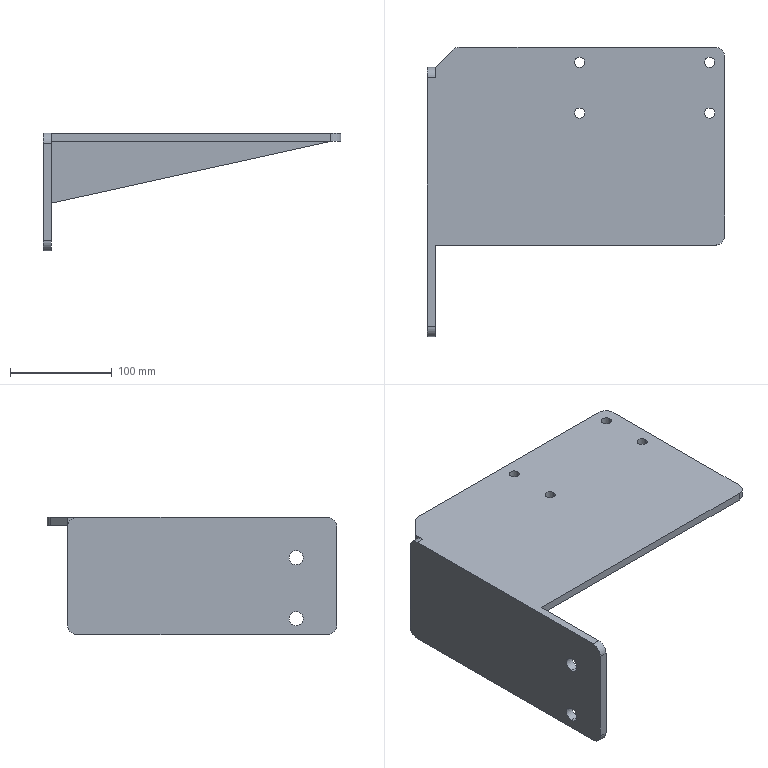Part | SolidWorks | features BaseBody 2 | 2 solids | 36 faces | box 293 x 285 x 116 mm | volume 750279 mm3 | cylinder 19 | plane 17 | commonest cylinder face diameters 10 x8 20 x7 14 x4
STEP:
#1=CARTESIAN_POINT('',(8.,40.,23.));
#2=VERTEX_POINT('',#1);
#3=CARTESIAN_POINT('',(8.,40.,9.));
#4=VERTEX_POINT('',#3);
#5=CARTESIAN_POINT('',(8.,40.,16.));
#6=DIRECTION('',(1.,0.,0.));
#7=DIRECTION('',(0.,1.,0.));
#8=AXIS2_PLACEMENT_3D('',#5,#6,#7);
#9=CIRCLE('',#8,7.);
#10=EDGE_CURVE('',#2,#4,#9,.T.);
#11=ORIENTED_EDGE('',*,*,#10,.T.);
#12=CARTESIAN_POINT('',(0.,40.,9.));
#13=VERTEX_POINT('',#12);
#14=CARTESIAN_POINT('',(8.,40.,9.));
#15=DIRECTION('',(-1.,0.,0.));
#16=VECTOR('',#15,1000.);
#17=LINE('',#14,#16);
#18=EDGE_CURVE('',#4,#13,#17,.T.);
#19=ORIENTED_EDGE('',*,*,#18,.T.);
#20=CARTESIAN_POINT('',(0.,40.,23.));
#21=VERTEX_POINT('',#20);
#22=CARTESIAN_POINT('',(0.,40.,16.));
#23=DIRECTION('',(1.,0.,0.));
#24=DIRECTION('',(0.,1.,0.));
#25=AXIS2_PLACEMENT_3D('',#22,#23,#24);
#26=CIRCLE('',#25,7.);
#27=EDGE_CURVE('',#21,#13,#26,.T.);
#28=ORIENTED_EDGE('',*,*,#27,.F.);
#29=CARTESIAN_POINT('',(8.,40.,23.));
#30=DIRECTION('',(-1.,0.,0.));
#31=VECTOR('',#30,1000.);
#32=LINE('',#29,#31);
#33=EDGE_CURVE('',#2,#21,#32,.T.);
#34=ORIENTED_EDGE('',*,*,#33,.F.);
#35=EDGE_LOOP('',(#11,#19,#28,#34));
#36=FACE_OUTER_BOUND('',#35,.T.);
#37=CARTESIAN_POINT('',(8.,40.,16.));
#38=DIRECTION('',(-1.,0.,0.));
#39=DIRECTION('',(0.,0.,1.));
#40=AXIS2_PLACEMENT_3D('',#37,#38,#39);
#41=CYLINDRICAL_SURFACE('',#40,7.);
#42=ADVANCED_FACE('',(#36),#41,.F.);
#43=CARTESIAN_POINT('',(8.,40.,83.));
#44=VERTEX_POINT('',#43);
#45=CARTESIAN_POINT('',(8.,40.,69.));
#46=VERTEX_POINT('',#45);
#47=CARTESIAN_POINT('',(8.,40.,76.));
#48=DIRECTION('',(1.,0.,0.));
#49=DIRECTION('',(0.,1.,0.));
#50=AXIS2_PLACEMENT_3D('',#47,#48,#49);
#51=CIRCLE('',#50,7.);
#52=EDGE_CURVE('',#44,#46,#51,.T.);
#53=ORIENTED_EDGE('',*,*,#52,.T.);
#54=CARTESIAN_POINT('',(0.,40.,69.));
#55=VERTEX_POINT('',#54);
#56=CARTESIAN_POINT('',(8.,40.,69.));
#57=DIRECTION('',(-1.,0.,0.));
#58=VECTOR('',#57,1000.);
#59=LINE('',#56,#58);
#60=EDGE_CURVE('',#46,#55,#59,.T.);
#61=ORIENTED_EDGE('',*,*,#60,.T.);
#62=CARTESIAN_POINT('',(0.,40.,83.));
#63=VERTEX_POINT('',#62);
#64=CARTESIAN_POINT('',(0.,40.,76.));
#65=DIRECTION('',(1.,0.,0.));
#66=DIRECTION('',(0.,1.,0.));
#67=AXIS2_PLACEMENT_3D('',#64,#65,#66);
#68=CIRCLE('',#67,7.);
#69=EDGE_CURVE('',#63,#55,#68,.T.);
#70=ORIENTED_EDGE('',*,*,#69,.F.);
#71=CARTESIAN_POINT('',(8.,40.,83.));
#72=DIRECTION('',(-1.,0.,0.));
#73=VECTOR('',#72,1000.);
#74=LINE('',#71,#73);
#75=EDGE_CURVE('',#44,#63,#74,.T.);
#76=ORIENTED_EDGE('',*,*,#75,.F.);
#77=EDGE_LOOP('',(#53,#61,#70,#76));
#78=FACE_OUTER_BOUND('',#77,.T.);
#79=CARTESIAN_POINT('',(8.,40.,76.));
#80=DIRECTION('',(-1.,0.,0.));
#81=DIRECTION('',(0.,0.,1.));
#82=AXIS2_PLACEMENT_3D('',#79,#80,#81);
#83=CYLINDRICAL_SURFACE('',#82,7.);
#84=ADVANCED_FACE('',(#78),#83,.F.);
#85=CARTESIAN_POINT('',(273.,270.,116.));
#86=VERTEX_POINT('',#85);
#87=CARTESIAN_POINT('',(283.,270.,116.));
#88=VERTEX_POINT('',#87);
#89=CARTESIAN_POINT('',(278.,270.,116.));
#90=DIRECTION('',(0.,0.,1.));
#91=DIRECTION('',(0.,1.,0.));
#92=AXIS2_PLACEMENT_3D('',#89,#90,#91);
#93=CIRCLE('',#92,5.);
#94=EDGE_CURVE('',#86,#88,#93,.T.);
#95=ORIENTED_EDGE('',*,*,#94,.T.);
#96=CARTESIAN_POINT('',(283.,270.,108.));
#97=VERTEX_POINT('',#96);
#98=CARTESIAN_POINT('',(283.,270.,366.));
#99=DIRECTION('',(0.,0.,-1.));
#100=VECTOR('',#99,1000.);
#101=LINE('',#98,#100);
#102=EDGE_CURVE('',#88,#97,#101,.T.);
#103=ORIENTED_EDGE('',*,*,#102,.T.);
#104=CARTESIAN_POINT('',(273.,270.,108.));
#105=VERTEX_POINT('',#104);
#106=CARTESIAN_POINT('',(278.,270.,108.));
#107=DIRECTION('',(0.,0.,-1.));
#108=DIRECTION('',(0.,1.,0.));
#109=AXIS2_PLACEMENT_3D('',#106,#107,#108);
#110=CIRCLE('',#109,5.);
#111=EDGE_CURVE('',#97,#105,#110,.T.);
#112=ORIENTED_EDGE('',*,*,#111,.T.);
#113=CARTESIAN_POINT('',(273.,270.,366.));
#114=DIRECTION('',(0.,0.,-1.));
#115=VECTOR('',#114,1000.);
#116=LINE('',#113,#115);
#117=EDGE_CURVE('',#86,#105,#116,.T.);
#118=ORIENTED_EDGE('',*,*,#117,.F.);
#119=EDGE_LOOP('',(#95,#103,#112,#118));
#120=FACE_OUTER_BOUND('',#119,.T.);
#121=CARTESIAN_POINT('',(278.,270.,366.));
#122=DIRECTION('',(0.,0.,-1.));
#123=DIRECTION('',(-1.,0.,0.));
#124=AXIS2_PLACEMENT_3D('',#121,#122,#123);
#125=CYLINDRICAL_SURFACE('',#124,5.);
#126=ADVANCED_FACE('',(#120),#125,.F.);
#127=CARTESIAN_POINT('',(273.,220.,116.));
#128=VERTEX_POINT('',#127);
#129=CARTESIAN_POINT('',(283.,220.,116.));
#130=VERTEX_POINT('',#129);
#131=CARTESIAN_POINT('',(278.,220.,116.));
#132=DIRECTION('',(0.,0.,1.));
#133=DIRECTION('',(0.,1.,0.));
#134=AXIS2_PLACEMENT_3D('',#131,#132,#133);
#135=CIRCLE('',#134,5.);
#136=EDGE_CURVE('',#128,#130,#135,.T.);
#137=ORIENTED_EDGE('',*,*,#136,.T.);
#138=CARTESIAN_POINT('',(283.,220.,108.));
#139=VERTEX_POINT('',#138);
#140=CARTESIAN_POINT('',(283.,220.,366.));
#141=DIRECTION('',(0.,0.,-1.));
#142=VECTOR('',#141,1000.);
#143=LINE('',#140,#142);
#144=EDGE_CURVE('',#130,#139,#143,.T.);
#145=ORIENTED_EDGE('',*,*,#144,.T.);
#146=CARTESIAN_POINT('',(273.,220.,108.));
#147=VERTEX_POINT('',#146);
#148=CARTESIAN_POINT('',(278.,220.,108.));
#149=DIRECTION('',(0.,0.,-1.));
#150=DIRECTION('',(0.,1.,0.));
#151=AXIS2_PLACEMENT_3D('',#148,#149,#150);
#152=CIRCLE('',#151,5.);
#153=EDGE_CURVE('',#139,#147,#152,.T.);
#154=ORIENTED_EDGE('',*,*,#153,.T.);
#155=CARTESIAN_POINT('',(273.,220.,366.));
#156=DIRECTION('',(0.,0.,-1.));
#157=VECTOR('',#156,1000.);
#158=LINE('',#155,#157);
#159=EDGE_CURVE('',#128,#147,#158,.T.);
#160=ORIENTED_EDGE('',*,*,#159,.F.);
#161=EDGE_LOOP('',(#137,#145,#154,#160));
#162=FACE_OUTER_BOUND('',#161,.T.);
#163=CARTESIAN_POINT('',(278.,220.,366.));
#164=DIRECTION('',(0.,0.,-1.));
#165=DIRECTION('',(-1.,0.,0.));
#166=AXIS2_PLACEMENT_3D('',#163,#164,#165);
#167=CYLINDRICAL_SURFACE('',#166,5.);
#168=ADVANCED_FACE('',(#162),#167,.F.);
#169=CARTESIAN_POINT('',(145.,270.,116.));
#170=VERTEX_POINT('',#169);
#171=CARTESIAN_POINT('',(155.,270.,116.));
#172=VERTEX_POINT('',#171);
#173=CARTESIAN_POINT('',(150.,270.,116.));
#174=DIRECTION('',(0.,0.,1.));
#175=DIRECTION('',(0.,1.,0.));
#176=AXIS2_PLACEMENT_3D('',#173,#174,#175);
#177=CIRCLE('',#176,5.);
#178=EDGE_CURVE('',#170,#172,#177,.T.);
#179=ORIENTED_EDGE('',*,*,#178,.T.);
#180=CARTESIAN_POINT('',(155.,270.,108.));
#181=VERTEX_POINT('',#180);
#182=CARTESIAN_POINT('',(155.,270.,366.));
#183=DIRECTION('',(0.,0.,-1.));
#184=VECTOR('',#183,1000.);
#185=LINE('',#182,#184);
#186=EDGE_CURVE('',#172,#181,#185,.T.);
#187=ORIENTED_EDGE('',*,*,#186,.T.);
#188=CARTESIAN_POINT('',(145.,270.,108.));
#189=VERTEX_POINT('',#188);
#190=CARTESIAN_POINT('',(150.,270.,108.));
#191=DIRECTION('',(0.,0.,-1.));
#192=DIRECTION('',(0.,1.,0.));
#193=AXIS2_PLACEMENT_3D('',#190,#191,#192);
#194=CIRCLE('',#193,5.);
#195=EDGE_CURVE('',#181,#189,#194,.T.);
#196=ORIENTED_EDGE('',*,*,#195,.T.);
#197=CARTESIAN_POINT('',(145.,270.,366.));
#198=DIRECTION('',(0.,0.,-1.));
#199=VECTOR('',#198,1000.);
#200=LINE('',#197,#199);
#201=EDGE_CURVE('',#170,#189,#200,.T.);
#202=ORIENTED_EDGE('',*,*,#201,.F.);
#203=EDGE_LOOP('',(#179,#187,#196,#202));
#204=FACE_OUTER_BOUND('',#203,.T.);
#205=CARTESIAN_POINT('',(150.,270.,366.));
#206=DIRECTION('',(0.,0.,-1.));
#207=DIRECTION('',(-1.,0.,0.));
#208=AXIS2_PLACEMENT_3D('',#205,#206,#207);
#209=CYLINDRICAL_SURFACE('',#208,5.);
#210=ADVANCED_FACE('',(#204),#209,.F.);
#211=CARTESIAN_POINT('',(145.,220.,116.));
#212=VERTEX_POINT('',#211);
#213=CARTESIAN_POINT('',(155.,220.,116.));
#214=VERTEX_POINT('',#213);
#215=CARTESIAN_POINT('',(150.,220.,116.));
#216=DIRECTION('',(0.,0.,1.));
#217=DIRECTION('',(0.,1.,0.));
#218=AXIS2_PLACEMENT_3D('',#215,#216,#217);
#219=CIRCLE('',#218,5.);
#220=EDGE_CURVE('',#212,#214,#219,.T.);
#221=ORIENTED_EDGE('',*,*,#220,.T.);
#222=CARTESIAN_POINT('',(155.,220.,108.));
#223=VERTEX_POINT('',#222);
#224=CARTESIAN_POINT('',(155.,220.,366.));
#225=DIRECTION('',(0.,0.,-1.));
#226=VECTOR('',#225,1000.);
#227=LINE('',#224,#226);
#228=EDGE_CURVE('',#214,#223,#227,.T.);
#229=ORIENTED_EDGE('',*,*,#228,.T.);
#230=CARTESIAN_POINT('',(145.,220.,108.));
#231=VERTEX_POINT('',#230);
#232=CARTESIAN_POINT('',(150.,220.,108.));
#233=DIRECTION('',(0.,0.,-1.));
#234=DIRECTION('',(0.,1.,0.));
#235=AXIS2_PLACEMENT_3D('',#232,#233,#234);
#236=CIRCLE('',#235,5.);
#237=EDGE_CURVE('',#223,#231,#236,.T.);
#238=ORIENTED_EDGE('',*,*,#237,.T.);
#239=CARTESIAN_POINT('',(145.,220.,366.));
#240=DIRECTION('',(0.,0.,-1.));
#241=VECTOR('',#240,1000.);
#242=LINE('',#239,#241);
#243=EDGE_CURVE('',#212,#231,#242,.T.);
#244=ORIENTED_EDGE('',*,*,#243,.F.);
#245=EDGE_LOOP('',(#221,#229,#238,#244));
#246=FACE_OUTER_BOUND('',#245,.T.);
#247=CARTESIAN_POINT('',(150.,220.,366.));
#248=DIRECTION('',(0.,0.,-1.));
#249=DIRECTION('',(-1.,0.,0.));
#250=AXIS2_PLACEMENT_3D('',#247,#248,#249);
#251=CYLINDRICAL_SURFACE('',#250,5.);
#252=ADVANCED_FACE('',(#246),#251,.F.);
#253=CARTESIAN_POINT('',(25.071,282.071,108.));
#254=VERTEX_POINT('',#253);
#255=CARTESIAN_POINT('',(32.142,285.,108.));
#256=VERTEX_POINT('',#255);
#257=CARTESIAN_POINT('',(32.142,275.,108.));
#258=DIRECTION('',(0.,0.,-1.));
#259=DIRECTION('',(0.,1.,0.));
#260=AXIS2_PLACEMENT_3D('',#257,#258,#259);
#261=CIRCLE('',#260,10.);
#262=EDGE_CURVE('',#254,#256,#261,.T.);
#263=ORIENTED_EDGE('',*,*,#262,.F.);
#264=CARTESIAN_POINT('',(25.071,282.071,116.));
#265=VERTEX_POINT('',#264);
#266=CARTESIAN_POINT('',(25.071,282.071,0.));
#267=DIRECTION('',(0.,0.,-1.));
#268=VECTOR('',#267,1000.);
#269=LINE('',#266,#268);
#270=EDGE_CURVE('',#265,#254,#269,.T.);
#271=ORIENTED_EDGE('',*,*,#270,.F.);
#272=CARTESIAN_POINT('',(32.142,285.,116.));
#273=VERTEX_POINT('',#272);
#274=CARTESIAN_POINT('',(32.142,275.,116.));
#275=DIRECTION('',(0.,0.,1.));
#276=DIRECTION('',(0.,1.,0.));
#277=AXIS2_PLACEMENT_3D('',#274,#275,#276);
#278=CIRCLE('',#277,10.);
#279=EDGE_CURVE('',#273,#265,#278,.T.);
#280=ORIENTED_EDGE('',*,*,#279,.F.);
#281=CARTESIAN_POINT('',(32.142,285.,116.));
#282=DIRECTION('',(0.,0.,1.));
#283=VECTOR('',#282,1000.);
#284=LINE('',#281,#283);
#285=EDGE_CURVE('',#256,#273,#284,.T.);
#286=ORIENTED_EDGE('',*,*,#285,.F.);
#287=EDGE_LOOP('',(#263,#271,#280,#286));
#288=FACE_OUTER_BOUND('',#287,.T.);
#289=CARTESIAN_POINT('',(32.142,275.,116.));
#290=DIRECTION('',(0.,0.,-1.));
#291=DIRECTION('',(-1.,0.,0.));
#292=AXIS2_PLACEMENT_3D('',#289,#290,#291);
#293=CYLINDRICAL_SURFACE('',#292,10.);
#294=ADVANCED_FACE('',(#288),#293,.T.);
#295=CARTESIAN_POINT('',(8.,265.,116.));
#296=VERTEX_POINT('',#295);
#297=CARTESIAN_POINT('',(8.,265.,116.));
#298=DIRECTION('',(-0.7071,-0.7071,0.));
#299=VECTOR('',#298,1000.);
#300=LINE('',#297,#299);
#301=EDGE_CURVE('',#265,#296,#300,.T.);
#302=ORIENTED_EDGE('',*,*,#301,.F.);
#303=ORIENTED_EDGE('',*,*,#270,.T.);
#304=CARTESIAN_POINT('',(8.,265.,108.));
#305=VERTEX_POINT('',#304);
#306=CARTESIAN_POINT('',(160.5,417.5,108.));
#307=DIRECTION('',(0.7071,0.7071,0.));
#308=VECTOR('',#307,1000.);
#309=LINE('',#306,#308);
#310=EDGE_CURVE('',#305,#254,#309,.T.);
#311=ORIENTED_EDGE('',*,*,#310,.F.);
#312=CARTESIAN_POINT('',(8.,265.,0.));
#313=DIRECTION('',(0.,0.,-1.));
#314=VECTOR('',#313,1000.);
#315=LINE('',#312,#314);
#316=EDGE_CURVE('',#296,#305,#315,.T.);
#317=ORIENTED_EDGE('',*,*,#316,.F.);
#318=EDGE_LOOP('',(#302,#303,#311,#317));
#319=FACE_OUTER_BOUND('',#318,.T.);
#320=CARTESIAN_POINT('',(8.,265.,0.));
#321=DIRECTION('',(0.7071,-0.7071,0.));
#322=DIRECTION('',(0.,0.,-1.));
#323=AXIS2_PLACEMENT_3D('',#320,#321,#322);
#324=PLANE('',#323);
#325=ADVANCED_FACE('',(#319),#324,.F.);
#326=CARTESIAN_POINT('',(293.,100.,108.));
#327=VERTEX_POINT('',#326);
#328=CARTESIAN_POINT('',(283.,90.,108.));
#329=VERTEX_POINT('',#328);
#330=CARTESIAN_POINT('',(283.,100.,108.));
#331=DIRECTION('',(0.,0.,-1.));
#332=DIRECTION('',(0.,1.,0.));
#333=AXIS2_PLACEMENT_3D('',#330,#331,#332);
#334=CIRCLE('',#333,10.);
#335=EDGE_CURVE('',#327,#329,#334,.T.);
#336=ORIENTED_EDGE('',*,*,#335,.F.);
#337=CARTESIAN_POINT('',(293.,100.,116.));
#338=VERTEX_POINT('',#337);
#339=CARTESIAN_POINT('',(293.,100.,108.));
#340=DIRECTION('',(0.,0.,-1.));
#341=VECTOR('',#340,1000.);
#342=LINE('',#339,#341);
#343=EDGE_CURVE('',#338,#327,#342,.T.);
#344=ORIENTED_EDGE('',*,*,#343,.F.);
#345=CARTESIAN_POINT('',(283.,90.,116.));
#346=VERTEX_POINT('',#345);
#347=CARTESIAN_POINT('',(283.,100.,116.));
#348=DIRECTION('',(0.,0.,1.));
#349=DIRECTION('',(0.,1.,0.));
#350=AXIS2_PLACEMENT_3D('',#347,#348,#349);
#351=CIRCLE('',#350,10.);
#352=EDGE_CURVE('',#346,#338,#351,.T.);
#353=ORIENTED_EDGE('',*,*,#352,.F.);
#354=CARTESIAN_POINT('',(283.,90.,116.));
#355=DIRECTION('',(0.,0.,1.));
#356=VECTOR('',#355,1000.);
#357=LINE('',#354,#356);
#358=EDGE_CURVE('',#329,#346,#357,.T.);
#359=ORIENTED_EDGE('',*,*,#358,.F.);
#360=EDGE_LOOP('',(#336,#344,#353,#359));
#361=FACE_OUTER_BOUND('',#360,.T.);
#362=CARTESIAN_POINT('',(283.,100.,108.));
#363=DIRECTION('',(0.,0.,-1.));
#364=DIRECTION('',(-1.,0.,0.));
#365=AXIS2_PLACEMENT_3D('',#362,#363,#364);
#366=CYLINDRICAL_SURFACE('',#365,10.);
#367=ADVANCED_FACE('',(#361),#366,.T.);
#368=CARTESIAN_POINT('',(293.,275.,116.));
#369=VERTEX_POINT('',#368);
#370=CARTESIAN_POINT('',(283.,285.,116.));
#371=VERTEX_POINT('',#370);
#372=CARTESIAN_POINT('',(283.,275.,116.));
#373=DIRECTION('',(0.,0.,1.));
#374=DIRECTION('',(0.,1.,0.));
#375=AXIS2_PLACEMENT_3D('',#372,#373,#374);
#376=CIRCLE('',#375,10.);
#377=EDGE_CURVE('',#369,#371,#376,.T.);
#378=ORIENTED_EDGE('',*,*,#377,.F.);
#379=CARTESIAN_POINT('',(293.,275.,108.));
#380=VERTEX_POINT('',#379);
#381=CARTESIAN_POINT('',(293.,275.,116.));
#382=DIRECTION('',(0.,0.,1.));
#383=VECTOR('',#382,1000.);
#384=LINE('',#381,#383);
#385=EDGE_CURVE('',#380,#369,#384,.T.);
#386=ORIENTED_EDGE('',*,*,#385,.F.);
#387=CARTESIAN_POINT('',(283.,285.,108.));
#388=VERTEX_POINT('',#387);
#389=CARTESIAN_POINT('',(283.,275.,108.));
#390=DIRECTION('',(0.,0.,-1.));
#391=DIRECTION('',(0.,1.,0.));
#392=AXIS2_PLACEMENT_3D('',#389,#390,#391);
#393=CIRCLE('',#392,10.);
#394=EDGE_CURVE('',#388,#380,#393,.T.);
#395=ORIENTED_EDGE('',*,*,#394,.F.);
#396=CARTESIAN_POINT('',(283.,285.,108.));
#397=DIRECTION('',(0.,0.,-1.));
#398=VECTOR('',#397,1000.);
#399=LINE('',#396,#398);
#400=EDGE_CURVE('',#371,#388,#399,.T.);
#401=ORIENTED_EDGE('',*,*,#400,.F.);
#402=EDGE_LOOP('',(#378,#386,#395,#401));
#403=FACE_OUTER_BOUND('',#402,.T.);
#404=CARTESIAN_POINT('',(283.,275.,116.));
#405=DIRECTION('',(0.,0.,1.));
#406=DIRECTION('',(1.,0.,0.));
#407=AXIS2_PLACEMENT_3D('',#404,#405,#406);
#408=CYLINDRICAL_SURFACE('',#407,10.);
#409=ADVANCED_FACE('',(#403),#408,.T.);
#410=ORIENTED_EDGE('',*,*,#228,.F.);
#411=CARTESIAN_POINT('',(150.,220.,116.));
#412=DIRECTION('',(0.,0.,1.));
#413=DIRECTION('',(0.,1.,0.));
#414=AXIS2_PLACEMENT_3D('',#411,#412,#413);
#415=CIRCLE('',#414,5.);
#416=EDGE_CURVE('',#214,#212,#415,.T.);
#417=ORIENTED_EDGE('',*,*,#416,.T.);
#418=ORIENTED_EDGE('',*,*,#243,.T.);
#419=CARTESIAN_POINT('',(150.,220.,108.));
#420=DIRECTION('',(0.,0.,-1.));
#421=DIRECTION('',(0.,1.,0.));
#422=AXIS2_PLACEMENT_3D('',#419,#420,#421);
#423=CIRCLE('',#422,5.);
#424=EDGE_CURVE('',#231,#223,#423,.T.);
#425=ORIENTED_EDGE('',*,*,#424,.T.);
#426=EDGE_LOOP('',(#410,#417,#418,#425));
#427=FACE_OUTER_BOUND('',#426,.T.);
#428=CARTESIAN_POINT('',(150.,220.,366.));
#429=DIRECTION('',(0.,0.,-1.));
#430=DIRECTION('',(-1.,0.,0.));
#431=AXIS2_PLACEMENT_3D('',#428,#429,#430);
#432=CYLINDRICAL_SURFACE('',#431,5.);
#433=ADVANCED_FACE('',(#427),#432,.F.);
#434=ORIENTED_EDGE('',*,*,#186,.F.);
#435=CARTESIAN_POINT('',(150.,270.,116.));
#436=DIRECTION('',(0.,0.,1.));
#437=DIRECTION('',(0.,1.,0.));
#438=AXIS2_PLACEMENT_3D('',#435,#436,#437);
#439=CIRCLE('',#438,5.);
#440=EDGE_CURVE('',#172,#170,#439,.T.);
#441=ORIENTED_EDGE('',*,*,#440,.T.);
#442=ORIENTED_EDGE('',*,*,#201,.T.);
#443=CARTESIAN_POINT('',(150.,270.,108.));
#444=DIRECTION('',(0.,0.,-1.));
#445=DIRECTION('',(0.,1.,0.));
#446=AXIS2_PLACEMENT_3D('',#443,#444,#445);
#447=CIRCLE('',#446,5.);
#448=EDGE_CURVE('',#189,#181,#447,.T.);
#449=ORIENTED_EDGE('',*,*,#448,.T.);
#450=EDGE_LOOP('',(#434,#441,#442,#449));
#451=FACE_OUTER_BOUND('',#450,.T.);
#452=CARTESIAN_POINT('',(150.,270.,366.));
#453=DIRECTION('',(0.,0.,-1.));
#454=DIRECTION('',(-1.,0.,0.));
#455=AXIS2_PLACEMENT_3D('',#452,#453,#454);
#456=CYLINDRICAL_SURFACE('',#455,5.);
#457=ADVANCED_FACE('',(#451),#456,.F.);
#458=ORIENTED_EDGE('',*,*,#144,.F.);
#459=CARTESIAN_POINT('',(278.,220.,116.));
#460=DIRECTION('',(0.,0.,1.));
#461=DIRECTION('',(0.,1.,0.));
#462=AXIS2_PLACEMENT_3D('',#459,#460,#461);
#463=CIRCLE('',#462,5.);
#464=EDGE_CURVE('',#130,#128,#463,.T.);
#465=ORIENTED_EDGE('',*,*,#464,.T.);
#466=ORIENTED_EDGE('',*,*,#159,.T.);
#467=CARTESIAN_POINT('',(278.,220.,108.));
#468=DIRECTION('',(0.,0.,-1.));
#469=DIRECTION('',(0.,1.,0.));
#470=AXIS2_PLACEMENT_3D('',#467,#468,#469);
#471=CIRCLE('',#470,5.);
#472=EDGE_CURVE('',#147,#139,#471,.T.);
#473=ORIENTED_EDGE('',*,*,#472,.T.);
#474=EDGE_LOOP('',(#458,#465,#466,#473));
#475=FACE_OUTER_BOUND('',#474,.T.);
#476=CARTESIAN_POINT('',(278.,220.,366.));
#477=DIRECTION('',(0.,0.,-1.));
#478=DIRECTION('',(-1.,0.,0.));
#479=AXIS2_PLACEMENT_3D('',#476,#477,#478);
#480=CYLINDRICAL_SURFACE('',#479,5.);
#481=ADVANCED_FACE('',(#475),#480,.F.);
#482=ORIENTED_EDGE('',*,*,#102,.F.);
#483=CARTESIAN_POINT('',(278.,270.,116.));
#484=DIRECTION('',(0.,0.,1.));
#485=DIRECTION('',(0.,1.,0.));
#486=AXIS2_PLACEMENT_3D('',#483,#484,#485);
#487=CIRCLE('',#486,5.);
#488=EDGE_CURVE('',#88,#86,#487,.T.);
#489=ORIENTED_EDGE('',*,*,#488,.T.);
#490=ORIENTED_EDGE('',*,*,#117,.T.);
#491=CARTESIAN_POINT('',(278.,270.,108.));
#492=DIRECTION('',(0.,0.,-1.));
#493=DIRECTION('',(0.,1.,0.));
#494=AXIS2_PLACEMENT_3D('',#491,#492,#493);
#495=CIRCLE('',#494,5.);
#496=EDGE_CURVE('',#105,#97,#495,.T.);
#497=ORIENTED_EDGE('',*,*,#496,.T.);
#498=EDGE_LOOP('',(#482,#489,#490,#497));
#499=FACE_OUTER_BOUND('',#498,.T.);
#500=CARTESIAN_POINT('',(278.,270.,366.));
#501=DIRECTION('',(0.,0.,-1.));
#502=DIRECTION('',(-1.,0.,0.));
#503=AXIS2_PLACEMENT_3D('',#500,#501,#502);
#504=CYLINDRICAL_SURFACE('',#503,5.);
#505=ADVANCED_FACE('',(#499),#504,.F.);
#506=CARTESIAN_POINT('',(8.,255.,116.));
#507=VERTEX_POINT('',#506);
#508=CARTESIAN_POINT('',(8.,90.,116.));
#509=DIRECTION('',(0.,1.,0.));
#510=VECTOR('',#509,1000.);
#511=LINE('',#508,#510);
#512=EDGE_CURVE('',#507,#296,#511,.T.);
#513=ORIENTED_EDGE('',*,*,#512,.T.);
#514=ORIENTED_EDGE('',*,*,#316,.T.);
#515=CARTESIAN_POINT('',(8.,264.798,108.));
#516=VERTEX_POINT('',#515);
#517=CARTESIAN_POINT('',(8.,285.,108.));
#518=DIRECTION('',(0.,-1.,0.));
#519=VECTOR('',#518,1000.);
#520=LINE('',#517,#519);
#521=EDGE_CURVE('',#305,#516,#520,.T.);
#522=ORIENTED_EDGE('',*,*,#521,.T.);
#523=CARTESIAN_POINT('',(8.,255.,106.));
#524=DIRECTION('',(1.,0.,0.));
#525=DIRECTION('',(0.,1.,0.));
#526=AXIS2_PLACEMENT_3D('',#523,#524,#525);
#527=CIRCLE('',#526,10.);
#528=EDGE_CURVE('',#516,#507,#527,.T.);
#529=ORIENTED_EDGE('',*,*,#528,.T.);
#530=EDGE_LOOP('',(#513,#514,#522,#529));
#531=FACE_OUTER_BOUND('',#530,.T.);
#532=CARTESIAN_POINT('',(8.,0.,0.));
#533=DIRECTION('',(-1.,0.,0.));
#534=DIRECTION('',(0.,0.,1.));
#535=AXIS2_PLACEMENT_3D('',#532,#533,#534);
#536=PLANE('',#535);
#537=ADVANCED_FACE('',(#531),#536,.T.);
#538=CARTESIAN_POINT('',(293.,285.,108.));
#539=DIRECTION('',(0.,-1.,0.));
#540=VECTOR('',#539,1000.);
#541=LINE('',#538,#540);
#542=EDGE_CURVE('',#380,#327,#541,.T.);
#543=ORIENTED_EDGE('',*,*,#542,.F.);
#544=ORIENTED_EDGE('',*,*,#385,.T.);
#545=CARTESIAN_POINT('',(293.,90.,116.));
#546=DIRECTION('',(0.,1.,0.));
#547=VECTOR('',#546,1000.);
#548=LINE('',#545,#547);
#549=EDGE_CURVE('',#338,#369,#548,.T.);
#550=ORIENTED_EDGE('',*,*,#549,.F.);
#551=ORIENTED_EDGE('',*,*,#343,.T.);
#552=EDGE_LOOP('',(#543,#544,#550,#551));
#553=FACE_OUTER_BOUND('',#552,.T.);
#554=CARTESIAN_POINT('',(293.,0.,0.));
#555=DIRECTION('',(-1.,0.,0.));
#556=DIRECTION('',(0.,0.,1.));
#557=AXIS2_PLACEMENT_3D('',#554,#555,#556);
#558=PLANE('',#557);
#559=ADVANCED_FACE('',(#553),#558,.F.);
#560=ORIENTED_EDGE('',*,*,#310,.T.);
#561=ORIENTED_EDGE('',*,*,#262,.T.);
#562=CARTESIAN_POINT('',(293.,285.,108.));
#563=DIRECTION('',(-1.,0.,0.));
#564=VECTOR('',#563,1000.);
#565=LINE('',#562,#564);
#566=EDGE_CURVE('',#388,#256,#565,.T.);
#567=ORIENTED_EDGE('',*,*,#566,.F.);
#568=ORIENTED_EDGE('',*,*,#394,.T.);
#569=ORIENTED_EDGE('',*,*,#542,.T.);
#570=ORIENTED_EDGE('',*,*,#335,.T.);
#571=CARTESIAN_POINT('',(8.,90.,108.));
#572=VERTEX_POINT('',#571);
#573=CARTESIAN_POINT('',(293.,90.,108.));
#574=DIRECTION('',(-1.,0.,0.));
#575=VECTOR('',#574,1000.);
#576=LINE('',#573,#575);
#577=EDGE_CURVE('',#329,#572,#576,.T.);
#578=ORIENTED_EDGE('',*,*,#577,.T.);
#579=CARTESIAN_POINT('',(8.,285.,108.));
#580=DIRECTION('',(0.,-1.,0.));
#581=VECTOR('',#580,1000.);
#582=LINE('',#579,#581);
#583=EDGE_CURVE('',#516,#572,#582,.T.);
#584=ORIENTED_EDGE('',*,*,#583,.F.);
#585=ORIENTED_EDGE('',*,*,#521,.F.);
#586=EDGE_LOOP('',(#560,#561,#567,#568,#569,#570,#578,#584,#585));
#587=FACE_OUTER_BOUND('',#586,.T.);
#588=ORIENTED_EDGE('',*,*,#496,.F.);
#589=ORIENTED_EDGE('',*,*,#111,.F.);
#590=EDGE_LOOP('',(#588,#589));
#591=FACE_BOUND('',#590,.T.);
#592=ORIENTED_EDGE('',*,*,#472,.F.);
#593=ORIENTED_EDGE('',*,*,#153,.F.);
#594=EDGE_LOOP('',(#592,#593));
#595=FACE_BOUND('',#594,.T.);
#596=ORIENTED_EDGE('',*,*,#448,.F.);
#597=ORIENTED_EDGE('',*,*,#195,.F.);
#598=EDGE_LOOP('',(#596,#597));
#599=FACE_BOUND('',#598,.T.);
#600=ORIENTED_EDGE('',*,*,#424,.F.);
#601=ORIENTED_EDGE('',*,*,#237,.F.);
#602=EDGE_LOOP('',(#600,#601));
#603=FACE_BOUND('',#602,.T.);
#604=CARTESIAN_POINT('',(293.,285.,108.));
#605=DIRECTION('',(0.,0.,-1.));
#606=DIRECTION('',(-1.,0.,0.));
#607=AXIS2_PLACEMENT_3D('',#604,#605,#606);
#608=PLANE('',#607);
#609=ADVANCED_FACE('',(#587,#591,#595,#599,#603),#608,.T.);
#610=ORIENTED_EDGE('',*,*,#566,.T.);
#611=ORIENTED_EDGE('',*,*,#285,.T.);
#612=CARTESIAN_POINT('',(293.,285.,116.));
#613=DIRECTION('',(-1.,0.,0.));
#614=VECTOR('',#613,1000.);
#615=LINE('',#612,#614);
#616=EDGE_CURVE('',#371,#273,#615,.T.);
#617=ORIENTED_EDGE('',*,*,#616,.F.);
#618=ORIENTED_EDGE('',*,*,#400,.T.);
#619=EDGE_LOOP('',(#610,#611,#617,#618));
#620=FACE_OUTER_BOUND('',#619,.T.);
#621=CARTESIAN_POINT('',(293.,285.,116.));
#622=DIRECTION('',(0.,1.,0.));
#623=DIRECTION('',(1.,0.,0.));
#624=AXIS2_PLACEMENT_3D('',#621,#622,#623);
#625=PLANE('',#624);
#626=ADVANCED_FACE('',(#620),#625,.T.);
#627=ORIENTED_EDGE('',*,*,#577,.F.);
#628=ORIENTED_EDGE('',*,*,#358,.T.);
#629=CARTESIAN_POINT('',(8.,90.,116.));
#630=VERTEX_POINT('',#629);
#631=CARTESIAN_POINT('',(293.,90.,116.));
#632=DIRECTION('',(-1.,0.,0.));
#633=VECTOR('',#632,1000.);
#634=LINE('',#631,#633);
#635=EDGE_CURVE('',#346,#630,#634,.T.);
#636=ORIENTED_EDGE('',*,*,#635,.T.);
#637=CARTESIAN_POINT('',(8.,90.,108.));
#638=DIRECTION('',(0.,0.,1.));
#639=VECTOR('',#638,1000.);
#640=LINE('',#637,#639);
#641=EDGE_CURVE('',#572,#630,#640,.T.);
#642=ORIENTED_EDGE('',*,*,#641,.F.);
#643=EDGE_LOOP('',(#627,#628,#636,#642));
#644=FACE_OUTER_BOUND('',#643,.T.);
#645=CARTESIAN_POINT('',(293.,90.,108.));
#646=DIRECTION('',(0.,-1.,0.));
#647=DIRECTION('',(0.,0.,-1.));
#648=AXIS2_PLACEMENT_3D('',#645,#646,#647);
#649=PLANE('',#648);
#650=ADVANCED_FACE('',(#644),#649,.T.);
#651=ORIENTED_EDGE('',*,*,#69,.T.);
#652=CARTESIAN_POINT('',(0.,40.,76.));
#653=DIRECTION('',(1.,0.,0.));
#654=DIRECTION('',(0.,1.,0.));
#655=AXIS2_PLACEMENT_3D('',#652,#653,#654);
#656=CIRCLE('',#655,7.);
#657=EDGE_CURVE('',#55,#63,#656,.T.);
#658=ORIENTED_EDGE('',*,*,#657,.T.);
#659=EDGE_LOOP('',(#651,#658));
#660=FACE_BOUND('',#659,.T.);
#661=ORIENTED_EDGE('',*,*,#27,.T.);
#662=CARTESIAN_POINT('',(0.,40.,16.));
#663=DIRECTION('',(1.,0.,0.));
#664=DIRECTION('',(0.,1.,0.));
#665=AXIS2_PLACEMENT_3D('',#662,#663,#664);
#666=CIRCLE('',#665,7.);
#667=EDGE_CURVE('',#13,#21,#666,.T.);
#668=ORIENTED_EDGE('',*,*,#667,.T.);
#669=EDGE_LOOP('',(#661,#668));
#670=FACE_BOUND('',#669,.T.);
#671=CARTESIAN_POINT('',(0.,0.,106.));
#672=VERTEX_POINT('',#671);
#673=CARTESIAN_POINT('',(0.,0.,10.));
#674=VERTEX_POINT('',#673);
#675=CARTESIAN_POINT('',(0.,0.,106.));
#676=DIRECTION('',(0.,0.,-1.));
#677=VECTOR('',#676,1000.);
#678=LINE('',#675,#677);
#679=EDGE_CURVE('',#672,#674,#678,.T.);
#680=ORIENTED_EDGE('',*,*,#679,.F.);
#681=CARTESIAN_POINT('',(0.,10.,116.));
#682=VERTEX_POINT('',#681);
#683=CARTESIAN_POINT('',(0.,10.,106.));
#684=DIRECTION('',(1.,0.,0.));
#685=DIRECTION('',(0.,1.,0.));
#686=AXIS2_PLACEMENT_3D('',#683,#684,#685);
#687=CIRCLE('',#686,10.);
#688=EDGE_CURVE('',#682,#672,#687,.T.);
#689=ORIENTED_EDGE('',*,*,#688,.F.);
#690=CARTESIAN_POINT('',(0.,255.,116.));
#691=VERTEX_POINT('',#690);
#692=CARTESIAN_POINT('',(0.,255.,116.));
#693=DIRECTION('',(0.,-1.,0.));
#694=VECTOR('',#693,1000.);
#695=LINE('',#692,#694);
#696=EDGE_CURVE('',#691,#682,#695,.T.);
#697=ORIENTED_EDGE('',*,*,#696,.F.);
#698=CARTESIAN_POINT('',(0.,265.,106.));
#699=VERTEX_POINT('',#698);
#700=CARTESIAN_POINT('',(0.,255.,106.));
#701=DIRECTION('',(1.,0.,0.));
#702=DIRECTION('',(0.,1.,0.));
#703=AXIS2_PLACEMENT_3D('',#700,#701,#702);
#704=CIRCLE('',#703,10.);
#705=EDGE_CURVE('',#699,#691,#704,.T.);
#706=ORIENTED_EDGE('',*,*,#705,.F.);
#707=CARTESIAN_POINT('',(0.,265.,10.));
#708=VERTEX_POINT('',#707);
#709=CARTESIAN_POINT('',(0.,265.,10.));
#710=DIRECTION('',(0.,0.,1.));
#711=VECTOR('',#710,1000.);
#712=LINE('',#709,#711);
#713=EDGE_CURVE('',#708,#699,#712,.T.);
#714=ORIENTED_EDGE('',*,*,#713,.F.);
#715=CARTESIAN_POINT('',(0.,255.,0.));
#716=VERTEX_POINT('',#715);
#717=CARTESIAN_POINT('',(0.,255.,10.));
#718=DIRECTION('',(1.,0.,0.));
#719=DIRECTION('',(0.,1.,0.));
#720=AXIS2_PLACEMENT_3D('',#717,#718,#719);
#721=CIRCLE('',#720,10.);
#722=EDGE_CURVE('',#716,#708,#721,.T.);
#723=ORIENTED_EDGE('',*,*,#722,.F.);
#724=CARTESIAN_POINT('',(0.,10.,0.));
#725=VERTEX_POINT('',#724);
#726=CARTESIAN_POINT('',(0.,10.,0.));
#727=DIRECTION('',(0.,1.,0.));
#728=VECTOR('',#727,1000.);
#729=LINE('',#726,#728);
#730=EDGE_CURVE('',#725,#716,#729,.T.);
#731=ORIENTED_EDGE('',*,*,#730,.F.);
#732=CARTESIAN_POINT('',(0.,10.,10.));
#733=DIRECTION('',(1.,0.,0.));
#734=DIRECTION('',(0.,1.,0.));
#735=AXIS2_PLACEMENT_3D('',#732,#733,#734);
#736=CIRCLE('',#735,10.);
#737=EDGE_CURVE('',#674,#725,#736,.T.);
#738=ORIENTED_EDGE('',*,*,#737,.F.);
#739=EDGE_LOOP('',(#680,#689,#697,#706,#714,#723,#731,#738));
#740=FACE_OUTER_BOUND('',#739,.T.);
#741=CARTESIAN_POINT('',(0.,10.,10.));
#742=DIRECTION('',(1.,0.,0.));
#743=DIRECTION('',(0.,1.,0.));
#744=AXIS2_PLACEMENT_3D('',#741,#742,#743);
#745=PLANE('',#744);
#746=ADVANCED_FACE('',(#660,#670,#740),#745,.F.);
#747=ORIENTED_EDGE('',*,*,#60,.F.);
#748=CARTESIAN_POINT('',(8.,40.,76.));
#749=DIRECTION('',(1.,0.,0.));
#750=DIRECTION('',(0.,1.,0.));
#751=AXIS2_PLACEMENT_3D('',#748,#749,#750);
#752=CIRCLE('',#751,7.);
#753=EDGE_CURVE('',#46,#44,#752,.T.);
#754=ORIENTED_EDGE('',*,*,#753,.T.);
#755=ORIENTED_EDGE('',*,*,#75,.T.);
#756=ORIENTED_EDGE('',*,*,#657,.F.);
#757=EDGE_LOOP('',(#747,#754,#755,#756));
#758=FACE_OUTER_BOUND('',#757,.T.);
#759=CARTESIAN_POINT('',(8.,40.,76.));
#760=DIRECTION('',(-1.,0.,0.));
#761=DIRECTION('',(0.,0.,1.));
#762=AXIS2_PLACEMENT_3D('',#759,#760,#761);
#763=CYLINDRICAL_SURFACE('',#762,7.);
#764=ADVANCED_FACE('',(#758),#763,.F.);
#765=ORIENTED_EDGE('',*,*,#688,.T.);
#766=CARTESIAN_POINT('',(8.,0.,106.));
#767=VERTEX_POINT('',#766);
#768=CARTESIAN_POINT('',(8.,0.,106.));
#769=DIRECTION('',(-1.,0.,0.));
#770=VECTOR('',#769,1000.);
#771=LINE('',#768,#770);
#772=EDGE_CURVE('',#767,#672,#771,.T.);
#773=ORIENTED_EDGE('',*,*,#772,.F.);
#774=CARTESIAN_POINT('',(8.,10.,116.));
#775=VERTEX_POINT('',#774);
#776=CARTESIAN_POINT('',(8.,10.,106.));
#777=DIRECTION('',(1.,0.,0.));
#778=DIRECTION('',(0.,1.,0.));
#779=AXIS2_PLACEMENT_3D('',#776,#777,#778);
#780=CIRCLE('',#779,10.);
#781=EDGE_CURVE('',#775,#767,#780,.T.);
#782=ORIENTED_EDGE('',*,*,#781,.F.);
#783=CARTESIAN_POINT('',(8.,10.,116.));
#784=DIRECTION('',(-1.,0.,0.));
#785=VECTOR('',#784,1000.);
#786=LINE('',#783,#785);
#787=EDGE_CURVE('',#775,#682,#786,.T.);
#788=ORIENTED_EDGE('',*,*,#787,.T.);
#789=EDGE_LOOP('',(#765,#773,#782,#788));
#790=FACE_OUTER_BOUND('',#789,.T.);
#791=CARTESIAN_POINT('',(8.,10.,106.));
#792=DIRECTION('',(-1.,0.,0.));
#793=DIRECTION('',(0.,0.,1.));
#794=AXIS2_PLACEMENT_3D('',#791,#792,#793);
#795=CYLINDRICAL_SURFACE('',#794,10.);
#796=ADVANCED_FACE('',(#790),#795,.T.);
#797=ORIENTED_EDGE('',*,*,#18,.F.);
#798=CARTESIAN_POINT('',(8.,40.,16.));
#799=DIRECTION('',(1.,0.,0.));
#800=DIRECTION('',(0.,1.,0.));
#801=AXIS2_PLACEMENT_3D('',#798,#799,#800);
#802=CIRCLE('',#801,7.);
#803=EDGE_CURVE('',#4,#2,#802,.T.);
#804=ORIENTED_EDGE('',*,*,#803,.T.);
#805=ORIENTED_EDGE('',*,*,#33,.T.);
#806=ORIENTED_EDGE('',*,*,#667,.F.);
#807=EDGE_LOOP('',(#797,#804,#805,#806));
#808=FACE_OUTER_BOUND('',#807,.T.);
#809=CARTESIAN_POINT('',(8.,40.,16.));
#810=DIRECTION('',(-1.,0.,0.));
#811=DIRECTION('',(0.,0.,1.));
#812=AXIS2_PLACEMENT_3D('',#809,#810,#811);
#813=CYLINDRICAL_SURFACE('',#812,7.);
#814=ADVANCED_FACE('',(#808),#813,.F.);
#815=ORIENTED_EDGE('',*,*,#616,.T.);
#816=ORIENTED_EDGE('',*,*,#279,.T.);
#817=ORIENTED_EDGE('',*,*,#301,.T.);
#818=ORIENTED_EDGE('',*,*,#512,.F.);
#819=CARTESIAN_POINT('',(8.,255.,116.));
#820=DIRECTION('',(-1.,0.,0.));
#821=VECTOR('',#820,1000.);
#822=LINE('',#819,#821);
#823=EDGE_CURVE('',#507,#691,#822,.T.);
#824=ORIENTED_EDGE('',*,*,#823,.T.);
#825=ORIENTED_EDGE('',*,*,#696,.T.);
#826=ORIENTED_EDGE('',*,*,#787,.F.);
#827=CARTESIAN_POINT('',(8.,255.,116.));
#828=DIRECTION('',(0.,-1.,0.));
#829=VECTOR('',#828,1000.);
#830=LINE('',#827,#829);
#831=EDGE_CURVE('',#630,#775,#830,.T.);
#832=ORIENTED_EDGE('',*,*,#831,.F.);
#833=ORIENTED_EDGE('',*,*,#635,.F.);
#834=ORIENTED_EDGE('',*,*,#352,.T.);
#835=ORIENTED_EDGE('',*,*,#549,.T.);
#836=ORIENTED_EDGE('',*,*,#377,.T.);
#837=EDGE_LOOP('',(#815,#816,#817,#818,#824,#825,#826,#832,#833,#834,#835,#836));
#838=FACE_OUTER_BOUND('',#837,.T.);
#839=ORIENTED_EDGE('',*,*,#94,.F.);
#840=ORIENTED_EDGE('',*,*,#488,.F.);
#841=EDGE_LOOP('',(#839,#840));
#842=FACE_BOUND('',#841,.T.);
#843=ORIENTED_EDGE('',*,*,#136,.F.);
#844=ORIENTED_EDGE('',*,*,#464,.F.);
#845=EDGE_LOOP('',(#843,#844));
#846=FACE_BOUND('',#845,.T.);
#847=ORIENTED_EDGE('',*,*,#178,.F.);
#848=ORIENTED_EDGE('',*,*,#440,.F.);
#849=EDGE_LOOP('',(#847,#848));
#850=FACE_BOUND('',#849,.T.);
#851=ORIENTED_EDGE('',*,*,#220,.F.);
#852=ORIENTED_EDGE('',*,*,#416,.F.);
#853=EDGE_LOOP('',(#851,#852));
#854=FACE_BOUND('',#853,.T.);
#855=CARTESIAN_POINT('',(8.,255.,116.));
#856=DIRECTION('',(0.,0.,-1.));
#857=DIRECTION('',(-1.,0.,0.));
#858=AXIS2_PLACEMENT_3D('',#855,#856,#857);
#859=PLANE('',#858);
#860=ADVANCED_FACE('',(#838,#842,#846,#850,#854),#859,.F.);
#861=ORIENTED_EDGE('',*,*,#705,.T.);
#862=ORIENTED_EDGE('',*,*,#823,.F.);
#863=ORIENTED_EDGE('',*,*,#528,.F.);
#864=CARTESIAN_POINT('',(8.,265.,106.));
#865=VERTEX_POINT('',#864);
#866=CARTESIAN_POINT('',(8.,255.,106.));
#867=DIRECTION('',(1.,0.,0.));
#868=DIRECTION('',(0.,1.,0.));
#869=AXIS2_PLACEMENT_3D('',#866,#867,#868);
#870=CIRCLE('',#869,10.);
#871=EDGE_CURVE('',#865,#516,#870,.T.);
#872=ORIENTED_EDGE('',*,*,#871,.F.);
#873=CARTESIAN_POINT('',(8.,265.,106.));
#874=DIRECTION('',(-1.,0.,0.));
#875=VECTOR('',#874,1000.);
#876=LINE('',#873,#875);
#877=EDGE_CURVE('',#865,#699,#876,.T.);
#878=ORIENTED_EDGE('',*,*,#877,.T.);
#879=EDGE_LOOP('',(#861,#862,#863,#872,#878));
#880=FACE_OUTER_BOUND('',#879,.T.);
#881=CARTESIAN_POINT('',(8.,255.,106.));
#882=DIRECTION('',(-1.,0.,0.));
#883=DIRECTION('',(0.,0.,1.));
#884=AXIS2_PLACEMENT_3D('',#881,#882,#883);
#885=CYLINDRICAL_SURFACE('',#884,10.);
#886=ADVANCED_FACE('',(#880),#885,.T.);
#887=ORIENTED_EDGE('',*,*,#713,.T.);
#888=ORIENTED_EDGE('',*,*,#877,.F.);
#889=CARTESIAN_POINT('',(8.,265.,10.));
#890=VERTEX_POINT('',#889);
#891=CARTESIAN_POINT('',(8.,265.,10.));
#892=DIRECTION('',(0.,0.,1.));
#893=VECTOR('',#892,1000.);
#894=LINE('',#891,#893);
#895=EDGE_CURVE('',#890,#865,#894,.T.);
#896=ORIENTED_EDGE('',*,*,#895,.F.);
#897=CARTESIAN_POINT('',(8.,265.,10.));
#898=DIRECTION('',(-1.,0.,0.));
#899=VECTOR('',#898,1000.);
#900=LINE('',#897,#899);
#901=EDGE_CURVE('',#890,#708,#900,.T.);
#902=ORIENTED_EDGE('',*,*,#901,.T.);
#903=EDGE_LOOP('',(#887,#888,#896,#902));
#904=FACE_OUTER_BOUND('',#903,.T.);
#905=CARTESIAN_POINT('',(8.,265.,10.));
#906=DIRECTION('',(0.,-1.,0.));
#907=DIRECTION('',(0.,0.,-1.));
#908=AXIS2_PLACEMENT_3D('',#905,#906,#907);
#909=PLANE('',#908);
#910=ADVANCED_FACE('',(#904),#909,.F.);
#911=ORIENTED_EDGE('',*,*,#722,.T.);
#912=ORIENTED_EDGE('',*,*,#901,.F.);
#913=CARTESIAN_POINT('',(8.,255.,0.));
#914=VERTEX_POINT('',#913);
#915=CARTESIAN_POINT('',(8.,255.,10.));
#916=DIRECTION('',(1.,0.,0.));
#917=DIRECTION('',(0.,1.,0.));
#918=AXIS2_PLACEMENT_3D('',#915,#916,#917);
#919=CIRCLE('',#918,10.);
#920=EDGE_CURVE('',#914,#890,#919,.T.);
#921=ORIENTED_EDGE('',*,*,#920,.F.);
#922=CARTESIAN_POINT('',(8.,255.,0.));
#923=DIRECTION('',(-1.,0.,0.));
#924=VECTOR('',#923,1000.);
#925=LINE('',#922,#924);
#926=EDGE_CURVE('',#914,#716,#925,.T.);
#927=ORIENTED_EDGE('',*,*,#926,.T.);
#928=EDGE_LOOP('',(#911,#912,#921,#927));
#929=FACE_OUTER_BOUND('',#928,.T.);
#930=CARTESIAN_POINT('',(8.,255.,10.));
#931=DIRECTION('',(-1.,0.,0.));
#932=DIRECTION('',(0.,0.,1.));
#933=AXIS2_PLACEMENT_3D('',#930,#931,#932);
#934=CYLINDRICAL_SURFACE('',#933,10.);
#935=ADVANCED_FACE('',(#929),#934,.T.);
#936=ORIENTED_EDGE('',*,*,#730,.T.);
#937=ORIENTED_EDGE('',*,*,#926,.F.);
#938=CARTESIAN_POINT('',(8.,10.,0.));
#939=VERTEX_POINT('',#938);
#940=CARTESIAN_POINT('',(8.,10.,0.));
#941=DIRECTION('',(0.,1.,0.));
#942=VECTOR('',#941,1000.);
#943=LINE('',#940,#942);
#944=EDGE_CURVE('',#939,#914,#943,.T.);
#945=ORIENTED_EDGE('',*,*,#944,.F.);
#946=CARTESIAN_POINT('',(8.,10.,0.));
#947=DIRECTION('',(-1.,0.,0.));
#948=VECTOR('',#947,1000.);
#949=LINE('',#946,#948);
#950=EDGE_CURVE('',#939,#725,#949,.T.);
#951=ORIENTED_EDGE('',*,*,#950,.T.);
#952=EDGE_LOOP('',(#936,#937,#945,#951));
#953=FACE_OUTER_BOUND('',#952,.T.);
#954=CARTESIAN_POINT('',(8.,10.,0.));
#955=DIRECTION('',(0.,0.,1.));
#956=DIRECTION('',(1.,0.,0.));
#957=AXIS2_PLACEMENT_3D('',#954,#955,#956);
#958=PLANE('',#957);
#959=ADVANCED_FACE('',(#953),#958,.F.);
#960=ORIENTED_EDGE('',*,*,#737,.T.);
#961=ORIENTED_EDGE('',*,*,#950,.F.);
#962=CARTESIAN_POINT('',(8.,0.,10.));
#963=VERTEX_POINT('',#962);
#964=CARTESIAN_POINT('',(8.,10.,10.));
#965=DIRECTION('',(1.,0.,0.));
#966=DIRECTION('',(0.,1.,0.));
#967=AXIS2_PLACEMENT_3D('',#964,#965,#966);
#968=CIRCLE('',#967,10.);
#969=EDGE_CURVE('',#963,#939,#968,.T.);
#970=ORIENTED_EDGE('',*,*,#969,.F.);
#971=CARTESIAN_POINT('',(8.,0.,10.));
#972=DIRECTION('',(-1.,0.,0.));
#973=VECTOR('',#972,1000.);
#974=LINE('',#971,#973);
#975=EDGE_CURVE('',#963,#674,#974,.T.);
#976=ORIENTED_EDGE('',*,*,#975,.T.);
#977=EDGE_LOOP('',(#960,#961,#970,#976));
#978=FACE_OUTER_BOUND('',#977,.T.);
#979=CARTESIAN_POINT('',(8.,10.,10.));
#980=DIRECTION('',(-1.,0.,0.));
#981=DIRECTION('',(0.,0.,1.));
#982=AXIS2_PLACEMENT_3D('',#979,#980,#981);
#983=CYLINDRICAL_SURFACE('',#982,10.);
#984=ADVANCED_FACE('',(#978),#983,.T.);
#985=ORIENTED_EDGE('',*,*,#679,.T.);
#986=ORIENTED_EDGE('',*,*,#975,.F.);
#987=CARTESIAN_POINT('',(8.,0.,106.));
#988=DIRECTION('',(0.,0.,-1.));
#989=VECTOR('',#988,1000.);
#990=LINE('',#987,#989);
#991=EDGE_CURVE('',#767,#963,#990,.T.);
#992=ORIENTED_EDGE('',*,*,#991,.F.);
#993=ORIENTED_EDGE('',*,*,#772,.T.);
#994=EDGE_LOOP('',(#985,#986,#992,#993));
#995=FACE_OUTER_BOUND('',#994,.T.);
#996=CARTESIAN_POINT('',(8.,0.,106.));
#997=DIRECTION('',(0.,1.,0.));
#998=DIRECTION('',(0.,0.,-1.));
#999=AXIS2_PLACEMENT_3D('',#996,#997,#998);
#1000=PLANE('',#999);
#1001=ADVANCED_FACE('',(#995),#1000,.F.);
#1002=ORIENTED_EDGE('',*,*,#583,.T.);
#1003=ORIENTED_EDGE('',*,*,#641,.T.);
#1004=ORIENTED_EDGE('',*,*,#831,.T.);
#1005=ORIENTED_EDGE('',*,*,#781,.T.);
#1006=ORIENTED_EDGE('',*,*,#991,.T.);
#1007=ORIENTED_EDGE('',*,*,#969,.T.);
#1008=ORIENTED_EDGE('',*,*,#944,.T.);
#1009=ORIENTED_EDGE('',*,*,#920,.T.);
#1010=ORIENTED_EDGE('',*,*,#895,.T.);
#1011=ORIENTED_EDGE('',*,*,#871,.T.);
#1012=EDGE_LOOP('',(#1002,#1003,#1004,#1005,#1006,#1007,#1008,#1009,#1010,#1011));
#1013=FACE_OUTER_BOUND('',#1012,.T.);
#1014=ORIENTED_EDGE('',*,*,#52,.F.);
#1015=ORIENTED_EDGE('',*,*,#753,.F.);
#1016=EDGE_LOOP('',(#1014,#1015));
#1017=FACE_BOUND('',#1016,.T.);
#1018=ORIENTED_EDGE('',*,*,#10,.F.);
#1019=ORIENTED_EDGE('',*,*,#803,.F.);
#1020=EDGE_LOOP('',(#1018,#1019));
#1021=FACE_BOUND('',#1020,.T.);
#1022=CARTESIAN_POINT('',(8.,10.,10.));
#1023=DIRECTION('',(1.,0.,0.));
#1024=DIRECTION('',(0.,1.,0.));
#1025=AXIS2_PLACEMENT_3D('',#1022,#1023,#1024);
#1026=PLANE('',#1025);
#1027=ADVANCED_FACE('',(#1013,#1017,#1021),#1026,.T.);
#1028=CLOSED_SHELL('',(#42,#84,#126,#168,#210,#252,#294,#325,#367,#409,#433,#457,#481,#505,#537,#559,#609,#626,#650,#746,#764,#796,#814,#860,#886,#910,#935,#959,#984,#1001,#1027));
#1029=MANIFOLD_SOLID_BREP('',#1028);
#1030=CARTESIAN_POINT('',(8.,170.,108.));
#1031=VERTEX_POINT('',#1030);
#1032=CARTESIAN_POINT('',(8.,170.,46.979));
#1033=VERTEX_POINT('',#1032);
#1034=CARTESIAN_POINT('',(8.,170.,108.));
#1035=DIRECTION('',(0.,0.,-1.));
#1036=VECTOR('',#1035,1000.);
#1037=LINE('',#1034,#1036);
#1038=EDGE_CURVE('',#1031,#1033,#1037,.T.);
#1039=ORIENTED_EDGE('',*,*,#1038,.T.);
#1040=CARTESIAN_POINT('',(284.061,170.,108.));
#1041=VERTEX_POINT('',#1040);
#1042=CARTESIAN_POINT('',(8.,170.,46.979));
#1043=DIRECTION('',(0.9764,0.,0.2158));
#1044=VECTOR('',#1043,1000.);
#1045=LINE('',#1042,#1044);
#1046=EDGE_CURVE('',#1033,#1041,#1045,.T.);
#1047=ORIENTED_EDGE('',*,*,#1046,.T.);
#1048=CARTESIAN_POINT('',(284.061,170.,108.));
#1049=DIRECTION('',(-1.,0.,0.));
#1050=VECTOR('',#1049,1000.);
#1051=LINE('',#1048,#1050);
#1052=EDGE_CURVE('',#1041,#1031,#1051,.T.);
#1053=ORIENTED_EDGE('',*,*,#1052,.T.);
#1054=EDGE_LOOP('',(#1039,#1047,#1053));
#1055=FACE_OUTER_BOUND('',#1054,.T.);
#1056=CARTESIAN_POINT('',(0.,170.,0.));
#1057=DIRECTION('',(0.,1.,0.));
#1058=DIRECTION('',(1.,0.,0.));
#1059=AXIS2_PLACEMENT_3D('',#1056,#1057,#1058);
#1060=PLANE('',#1059);
#1061=ADVANCED_FACE('',(#1055),#1060,.F.);
#1062=CARTESIAN_POINT('',(8.,178.,108.));
#1063=VERTEX_POINT('',#1062);
#1064=CARTESIAN_POINT('',(8.,178.,46.979));
#1065=VERTEX_POINT('',#1064);
#1066=CARTESIAN_POINT('',(8.,178.,108.));
#1067=DIRECTION('',(0.,0.,-1.));
#1068=VECTOR('',#1067,1000.);
#1069=LINE('',#1066,#1068);
#1070=EDGE_CURVE('',#1063,#1065,#1069,.T.);
#1071=ORIENTED_EDGE('',*,*,#1070,.F.);
#1072=CARTESIAN_POINT('',(284.061,178.,108.));
#1073=VERTEX_POINT('',#1072);
#1074=CARTESIAN_POINT('',(284.061,178.,108.));
#1075=DIRECTION('',(-1.,0.,0.));
#1076=VECTOR('',#1075,1000.);
#1077=LINE('',#1074,#1076);
#1078=EDGE_CURVE('',#1073,#1063,#1077,.T.);
#1079=ORIENTED_EDGE('',*,*,#1078,.F.);
#1080=CARTESIAN_POINT('',(8.,178.,46.979));
#1081=DIRECTION('',(0.9764,0.,0.2158));
#1082=VECTOR('',#1081,1000.);
#1083=LINE('',#1080,#1082);
#1084=EDGE_CURVE('',#1065,#1073,#1083,.T.);
#1085=ORIENTED_EDGE('',*,*,#1084,.F.);
#1086=EDGE_LOOP('',(#1071,#1079,#1085));
#1087=FACE_OUTER_BOUND('',#1086,.T.);
#1088=CARTESIAN_POINT('',(0.,178.,0.));
#1089=DIRECTION('',(0.,1.,0.));
#1090=DIRECTION('',(1.,0.,0.));
#1091=AXIS2_PLACEMENT_3D('',#1088,#1089,#1090);
#1092=PLANE('',#1091);
#1093=ADVANCED_FACE('',(#1087),#1092,.T.);
#1094=ORIENTED_EDGE('',*,*,#1052,.F.);
#1095=CARTESIAN_POINT('',(284.061,178.,108.));
#1096=DIRECTION('',(0.,-1.,0.));
#1097=VECTOR('',#1096,1000.);
#1098=LINE('',#1095,#1097);
#1099=EDGE_CURVE('',#1073,#1041,#1098,.T.);
#1100=ORIENTED_EDGE('',*,*,#1099,.F.);
#1101=ORIENTED_EDGE('',*,*,#1078,.T.);
#1102=CARTESIAN_POINT('',(8.,178.,108.));
#1103=DIRECTION('',(0.,-1.,0.));
#1104=VECTOR('',#1103,1000.);
#1105=LINE('',#1102,#1104);
#1106=EDGE_CURVE('',#1063,#1031,#1105,.T.);
#1107=ORIENTED_EDGE('',*,*,#1106,.T.);
#1108=EDGE_LOOP('',(#1094,#1100,#1101,#1107));
#1109=FACE_OUTER_BOUND('',#1108,.T.);
#1110=CARTESIAN_POINT('',(284.061,178.,108.));
#1111=DIRECTION('',(0.,0.,1.));
#1112=DIRECTION('',(1.,0.,0.));
#1113=AXIS2_PLACEMENT_3D('',#1110,#1111,#1112);
#1114=PLANE('',#1113);
#1115=ADVANCED_FACE('',(#1109),#1114,.T.);
#1116=ORIENTED_EDGE('',*,*,#1046,.F.);
#1117=CARTESIAN_POINT('',(8.,178.,46.979));
#1118=DIRECTION('',(0.,-1.,0.));
#1119=VECTOR('',#1118,1000.);
#1120=LINE('',#1117,#1119);
#1121=EDGE_CURVE('',#1065,#1033,#1120,.T.);
#1122=ORIENTED_EDGE('',*,*,#1121,.F.);
#1123=ORIENTED_EDGE('',*,*,#1084,.T.);
#1124=ORIENTED_EDGE('',*,*,#1099,.T.);
#1125=EDGE_LOOP('',(#1116,#1122,#1123,#1124));
#1126=FACE_OUTER_BOUND('',#1125,.T.);
#1127=CARTESIAN_POINT('',(8.,178.,46.979));
#1128=DIRECTION('',(0.2158,0.,-0.9764));
#1129=DIRECTION('',(0.,-1.,0.));
#1130=AXIS2_PLACEMENT_3D('',#1127,#1128,#1129);
#1131=PLANE('',#1130);
#1132=ADVANCED_FACE('',(#1126),#1131,.T.);
#1133=ORIENTED_EDGE('',*,*,#1038,.F.);
#1134=ORIENTED_EDGE('',*,*,#1106,.F.);
#1135=ORIENTED_EDGE('',*,*,#1070,.T.);
#1136=ORIENTED_EDGE('',*,*,#1121,.T.);
#1137=EDGE_LOOP('',(#1133,#1134,#1135,#1136));
#1138=FACE_OUTER_BOUND('',#1137,.T.);
#1139=CARTESIAN_POINT('',(8.,178.,108.));
#1140=DIRECTION('',(-1.,0.,0.));
#1141=DIRECTION('',(0.,0.,1.));
#1142=AXIS2_PLACEMENT_3D('',#1139,#1140,#1141);
#1143=PLANE('',#1142);
#1144=ADVANCED_FACE('',(#1138),#1143,.T.);
#1145=CLOSED_SHELL('',(#1061,#1093,#1115,#1132,#1144));
#1146=MANIFOLD_SOLID_BREP('',#1145);
#1147=CARTESIAN_POINT('',(0.,0.,0.));
#1148=DIRECTION('',(0.,0.,1.));
#1149=DIRECTION('',(1.,0.,0.));
#1150=AXIS2_PLACEMENT_3D('',#1147,#1148,#1149);
#1151=(LENGTH_UNIT()NAMED_UNIT(*)SI_UNIT(.MILLI.,.METRE.));
#1152=UNCERTAINTY_MEASURE_WITH_UNIT(LENGTH_MEASURE(0.00001),#1151,'','');
#1153=(NAMED_UNIT(*)PLANE_ANGLE_UNIT()SI_UNIT($,.RADIAN.));
#1154=(NAMED_UNIT(*)SI_UNIT($,.STERADIAN.)SOLID_ANGLE_UNIT());
#1155=(GEOMETRIC_REPRESENTATION_CONTEXT(3)GLOBAL_UNCERTAINTY_ASSIGNED_CONTEXT((#1152))GLOBAL_UNIT_ASSIGNED_CONTEXT((#1151,#1153,#1154))REPRESENTATION_CONTEXT('',''));
#1156=ADVANCED_BREP_SHAPE_REPRESENTATION('',(#1029,#1146,#1150),#1155);